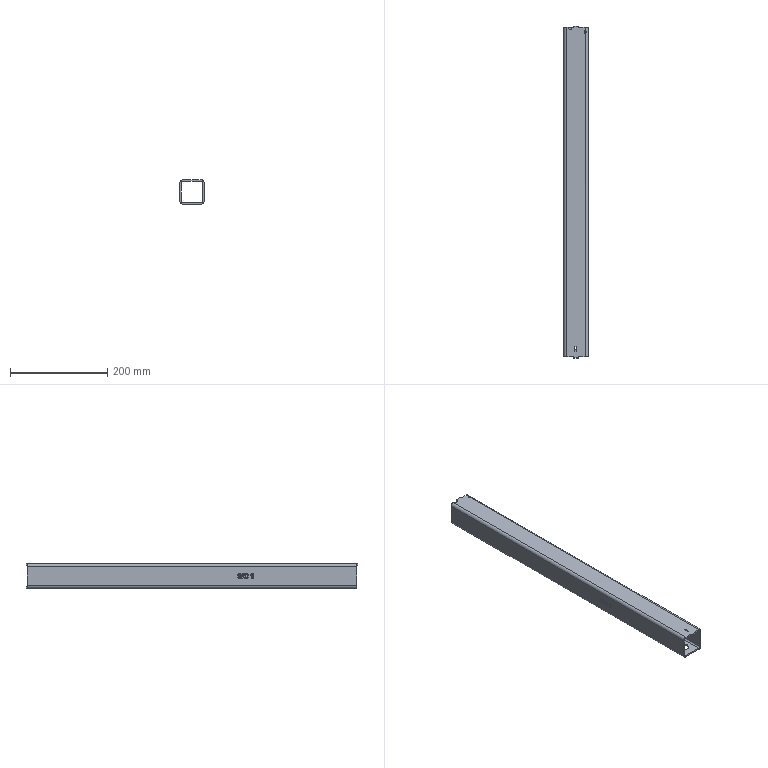Part | SolidWorks | features BaseBody 1 | 1 solid | 128 faces | box 50 x 682 x 50 mm | volume 361396 mm3 | plane 67 | spline 34 | cylinder 25 | cone 2 | commonest cylinder face diameters 20 x8 5.1 x6 6 x4 12 x4 4.2 x2 8 x1